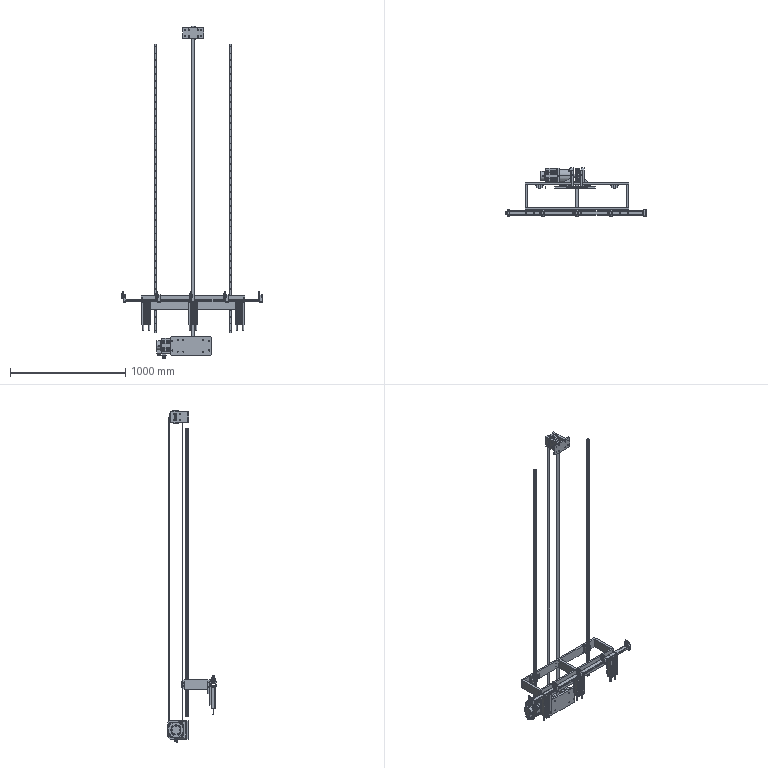Part | SolidWorks | features ReferencePattern 12, LocalLPattern 4, CompositeCurve 3 | 57 solids | 6232 faces | volume 15629653 mm3 | cylinder 2906 | plane 2316 | cone 796 | torus 106 | sphere 56 | spline 52 | commonest cylinder face diameters 2.5 x292 11 x246 6.6 x198 1.2 x173 1.6 x172 2 x112